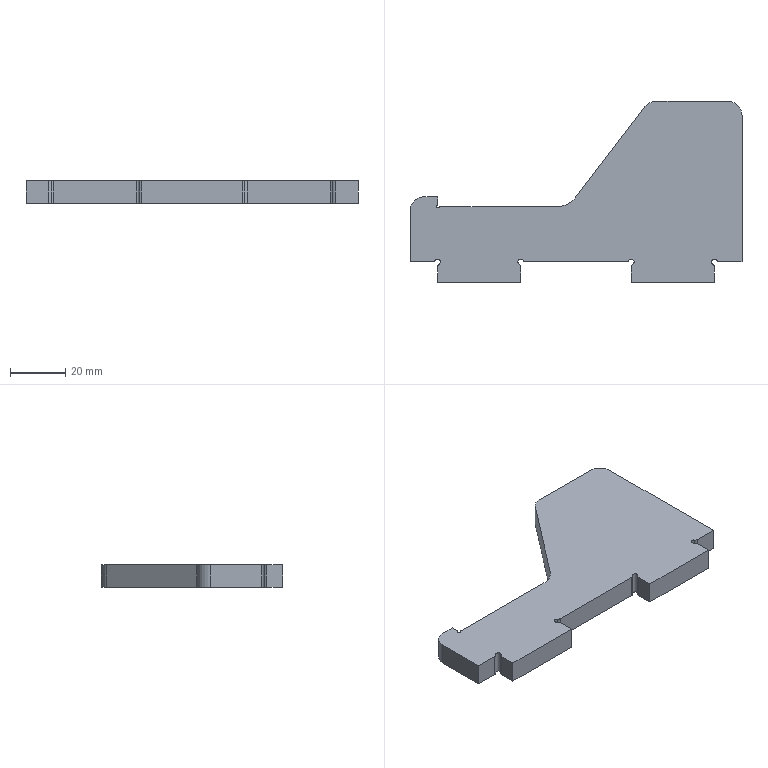Part | SolidWorks | features FlatPattern 1, SMBaseFlange 1, SheetMetal 1 | 1 solid | 39 faces | box 120 x 65.5 x 8 mm | volume 37548 mm3 | cylinder 21 | plane 18 | commonest cylinder face diameters 2 x16 10 x3 1 x1 16 x1
STEP:
#1=CARTESIAN_POINT('',(-85.366,-78.6,-8.));
#2=VERTEX_POINT('',#1);
#3=CARTESIAN_POINT('',(-83.5,-79.1,-8.));
#4=VERTEX_POINT('',#3);
#5=CARTESIAN_POINT('',(-84.5,-79.1,-8.));
#6=DIRECTION('',(0.,0.,-1.));
#7=DIRECTION('',(1.,0.,0.));
#8=AXIS2_PLACEMENT_3D('',#5,#6,#7);
#9=CIRCLE('',#8,1.);
#10=EDGE_CURVE('',#2,#4,#9,.T.);
#11=ORIENTED_EDGE('',*,*,#10,.T.);
#12=CARTESIAN_POINT('',(-83.5,-79.1,0.));
#13=VERTEX_POINT('',#12);
#14=CARTESIAN_POINT('',(-83.5,-79.1,-8.));
#15=DIRECTION('',(0.,0.,1.));
#16=VECTOR('',#15,1000.);
#17=LINE('',#14,#16);
#18=EDGE_CURVE('',#4,#13,#17,.T.);
#19=ORIENTED_EDGE('',*,*,#18,.T.);
#20=CARTESIAN_POINT('',(-85.366,-78.6,0.));
#21=VERTEX_POINT('',#20);
#22=CARTESIAN_POINT('',(-84.5,-79.1,0.));
#23=DIRECTION('',(0.,0.,-1.));
#24=DIRECTION('',(1.,0.,0.));
#25=AXIS2_PLACEMENT_3D('',#22,#23,#24);
#26=CIRCLE('',#25,1.);
#27=EDGE_CURVE('',#21,#13,#26,.T.);
#28=ORIENTED_EDGE('',*,*,#27,.F.);
#29=CARTESIAN_POINT('',(-85.366,-78.6,-8.));
#30=DIRECTION('',(0.,0.,1.));
#31=VECTOR('',#30,1000.);
#32=LINE('',#29,#31);
#33=EDGE_CURVE('',#2,#21,#32,.T.);
#34=ORIENTED_EDGE('',*,*,#33,.F.);
#35=EDGE_LOOP('',(#11,#19,#28,#34));
#36=FACE_OUTER_BOUND('',#35,.T.);
#37=CARTESIAN_POINT('',(-84.5,-79.1,-8.));
#38=DIRECTION('',(0.,0.,1.));
#39=DIRECTION('',(1.,0.,0.));
#40=AXIS2_PLACEMENT_3D('',#37,#38,#39);
#41=CYLINDRICAL_SURFACE('',#40,1.);
#42=ADVANCED_FACE('',(#36),#41,.F.);
#43=CARTESIAN_POINT('',(-15.366,-78.6,-8.));
#44=VERTEX_POINT('',#43);
#45=CARTESIAN_POINT('',(-13.5,-79.1,-8.));
#46=VERTEX_POINT('',#45);
#47=CARTESIAN_POINT('',(-14.5,-79.1,-8.));
#48=DIRECTION('',(0.,0.,-1.));
#49=DIRECTION('',(1.,0.,0.));
#50=AXIS2_PLACEMENT_3D('',#47,#48,#49);
#51=CIRCLE('',#50,1.);
#52=EDGE_CURVE('',#44,#46,#51,.T.);
#53=ORIENTED_EDGE('',*,*,#52,.T.);
#54=CARTESIAN_POINT('',(-13.5,-79.1,0.));
#55=VERTEX_POINT('',#54);
#56=CARTESIAN_POINT('',(-13.5,-79.1,-8.));
#57=DIRECTION('',(0.,0.,1.));
#58=VECTOR('',#57,1000.);
#59=LINE('',#56,#58);
#60=EDGE_CURVE('',#46,#55,#59,.T.);
#61=ORIENTED_EDGE('',*,*,#60,.T.);
#62=CARTESIAN_POINT('',(-15.366,-78.6,0.));
#63=VERTEX_POINT('',#62);
#64=CARTESIAN_POINT('',(-14.5,-79.1,0.));
#65=DIRECTION('',(0.,0.,-1.));
#66=DIRECTION('',(1.,0.,0.));
#67=AXIS2_PLACEMENT_3D('',#64,#65,#66);
#68=CIRCLE('',#67,1.);
#69=EDGE_CURVE('',#63,#55,#68,.T.);
#70=ORIENTED_EDGE('',*,*,#69,.F.);
#71=CARTESIAN_POINT('',(-15.366,-78.6,-8.));
#72=DIRECTION('',(0.,0.,1.));
#73=VECTOR('',#72,1000.);
#74=LINE('',#71,#73);
#75=EDGE_CURVE('',#44,#63,#74,.T.);
#76=ORIENTED_EDGE('',*,*,#75,.F.);
#77=EDGE_LOOP('',(#53,#61,#70,#76));
#78=FACE_OUTER_BOUND('',#77,.T.);
#79=CARTESIAN_POINT('',(-14.5,-79.1,-8.));
#80=DIRECTION('',(0.,0.,1.));
#81=DIRECTION('',(1.,0.,0.));
#82=AXIS2_PLACEMENT_3D('',#79,#80,#81);
#83=CYLINDRICAL_SURFACE('',#82,1.);
#84=ADVANCED_FACE('',(#78),#83,.F.);
#85=CARTESIAN_POINT('',(17.232,-79.1,0.));
#86=VERTEX_POINT('',#85);
#87=CARTESIAN_POINT('',(25.5,-79.1,0.));
#88=VERTEX_POINT('',#87);
#89=CARTESIAN_POINT('',(25.5,-79.1,0.));
#90=DIRECTION('',(1.,0.,0.));
#91=VECTOR('',#90,1000.);
#92=LINE('',#89,#91);
#93=EDGE_CURVE('',#86,#88,#92,.T.);
#94=ORIENTED_EDGE('',*,*,#93,.F.);
#95=CARTESIAN_POINT('',(17.232,-79.1,-8.));
#96=VERTEX_POINT('',#95);
#97=CARTESIAN_POINT('',(17.232,-79.1,-8.));
#98=DIRECTION('',(0.,0.,1.));
#99=VECTOR('',#98,1000.);
#100=LINE('',#97,#99);
#101=EDGE_CURVE('',#96,#86,#100,.T.);
#102=ORIENTED_EDGE('',*,*,#101,.F.);
#103=CARTESIAN_POINT('',(25.5,-79.1,-8.));
#104=VERTEX_POINT('',#103);
#105=CARTESIAN_POINT('',(25.5,-79.1,-8.));
#106=DIRECTION('',(1.,0.,0.));
#107=VECTOR('',#106,1000.);
#108=LINE('',#105,#107);
#109=EDGE_CURVE('',#96,#104,#108,.T.);
#110=ORIENTED_EDGE('',*,*,#109,.T.);
#111=CARTESIAN_POINT('',(25.5,-79.1,-8.));
#112=DIRECTION('',(0.,0.,1.));
#113=VECTOR('',#112,1000.);
#114=LINE('',#111,#113);
#115=EDGE_CURVE('',#104,#88,#114,.T.);
#116=ORIENTED_EDGE('',*,*,#115,.T.);
#117=EDGE_LOOP('',(#94,#102,#110,#116));
#118=FACE_OUTER_BOUND('',#117,.T.);
#119=CARTESIAN_POINT('',(25.5,-79.1,-8.));
#120=DIRECTION('',(0.,-1.,0.));
#121=DIRECTION('',(0.,0.,-1.));
#122=AXIS2_PLACEMENT_3D('',#119,#120,#121);
#123=PLANE('',#122);
#124=ADVANCED_FACE('',(#118),#123,.T.);
#125=CARTESIAN_POINT('',(16.366,-78.6,0.));
#126=VERTEX_POINT('',#125);
#127=CARTESIAN_POINT('',(17.232,-78.1,0.));
#128=DIRECTION('',(0.,0.,1.));
#129=DIRECTION('',(1.,0.,0.));
#130=AXIS2_PLACEMENT_3D('',#127,#128,#129);
#131=CIRCLE('',#130,1.);
#132=EDGE_CURVE('',#126,#86,#131,.T.);
#133=ORIENTED_EDGE('',*,*,#132,.F.);
#134=CARTESIAN_POINT('',(16.366,-78.6,-8.));
#135=VERTEX_POINT('',#134);
#136=CARTESIAN_POINT('',(16.366,-78.6,-8.));
#137=DIRECTION('',(0.,0.,1.));
#138=VECTOR('',#137,1000.);
#139=LINE('',#136,#138);
#140=EDGE_CURVE('',#135,#126,#139,.T.);
#141=ORIENTED_EDGE('',*,*,#140,.F.);
#142=CARTESIAN_POINT('',(17.232,-78.1,-8.));
#143=DIRECTION('',(0.,0.,1.));
#144=DIRECTION('',(1.,0.,0.));
#145=AXIS2_PLACEMENT_3D('',#142,#143,#144);
#146=CIRCLE('',#145,1.);
#147=EDGE_CURVE('',#135,#96,#146,.T.);
#148=ORIENTED_EDGE('',*,*,#147,.T.);
#149=ORIENTED_EDGE('',*,*,#101,.T.);
#150=EDGE_LOOP('',(#133,#141,#148,#149));
#151=FACE_OUTER_BOUND('',#150,.T.);
#152=CARTESIAN_POINT('',(17.232,-78.1,-8.));
#153=DIRECTION('',(0.,0.,1.));
#154=DIRECTION('',(1.,0.,0.));
#155=AXIS2_PLACEMENT_3D('',#152,#153,#154);
#156=CYLINDRICAL_SURFACE('',#155,1.);
#157=ADVANCED_FACE('',(#151),#156,.T.);
#158=CARTESIAN_POINT('',(15.,-79.966,0.));
#159=VERTEX_POINT('',#158);
#160=CARTESIAN_POINT('',(15.5,-79.1,0.));
#161=DIRECTION('',(0.,0.,-1.));
#162=DIRECTION('',(1.,0.,0.));
#163=AXIS2_PLACEMENT_3D('',#160,#161,#162);
#164=CIRCLE('',#163,1.);
#165=EDGE_CURVE('',#159,#126,#164,.T.);
#166=ORIENTED_EDGE('',*,*,#165,.F.);
#167=CARTESIAN_POINT('',(15.,-79.966,-8.));
#168=VERTEX_POINT('',#167);
#169=CARTESIAN_POINT('',(15.,-79.966,-8.));
#170=DIRECTION('',(0.,0.,1.));
#171=VECTOR('',#170,1000.);
#172=LINE('',#169,#171);
#173=EDGE_CURVE('',#168,#159,#172,.T.);
#174=ORIENTED_EDGE('',*,*,#173,.F.);
#175=CARTESIAN_POINT('',(15.5,-79.1,-8.));
#176=DIRECTION('',(0.,0.,-1.));
#177=DIRECTION('',(1.,0.,0.));
#178=AXIS2_PLACEMENT_3D('',#175,#176,#177);
#179=CIRCLE('',#178,1.);
#180=EDGE_CURVE('',#168,#135,#179,.T.);
#181=ORIENTED_EDGE('',*,*,#180,.T.);
#182=ORIENTED_EDGE('',*,*,#140,.T.);
#183=EDGE_LOOP('',(#166,#174,#181,#182));
#184=FACE_OUTER_BOUND('',#183,.T.);
#185=CARTESIAN_POINT('',(15.5,-79.1,-8.));
#186=DIRECTION('',(0.,0.,1.));
#187=DIRECTION('',(1.,0.,0.));
#188=AXIS2_PLACEMENT_3D('',#185,#186,#187);
#189=CYLINDRICAL_SURFACE('',#188,1.);
#190=ADVANCED_FACE('',(#184),#189,.F.);
#191=CARTESIAN_POINT('',(15.5,-80.832,0.));
#192=VERTEX_POINT('',#191);
#193=CARTESIAN_POINT('',(14.5,-80.832,0.));
#194=DIRECTION('',(0.,0.,1.));
#195=DIRECTION('',(-1.,0.,0.));
#196=AXIS2_PLACEMENT_3D('',#193,#194,#195);
#197=CIRCLE('',#196,1.);
#198=EDGE_CURVE('',#192,#159,#197,.T.);
#199=ORIENTED_EDGE('',*,*,#198,.F.);
#200=CARTESIAN_POINT('',(15.5,-80.832,-8.));
#201=VERTEX_POINT('',#200);
#202=CARTESIAN_POINT('',(15.5,-80.832,-8.));
#203=DIRECTION('',(0.,0.,1.));
#204=VECTOR('',#203,1000.);
#205=LINE('',#202,#204);
#206=EDGE_CURVE('',#201,#192,#205,.T.);
#207=ORIENTED_EDGE('',*,*,#206,.F.);
#208=CARTESIAN_POINT('',(14.5,-80.832,-8.));
#209=DIRECTION('',(0.,0.,1.));
#210=DIRECTION('',(-1.,0.,0.));
#211=AXIS2_PLACEMENT_3D('',#208,#209,#210);
#212=CIRCLE('',#211,1.);
#213=EDGE_CURVE('',#201,#168,#212,.T.);
#214=ORIENTED_EDGE('',*,*,#213,.T.);
#215=ORIENTED_EDGE('',*,*,#173,.T.);
#216=EDGE_LOOP('',(#199,#207,#214,#215));
#217=FACE_OUTER_BOUND('',#216,.T.);
#218=CARTESIAN_POINT('',(14.5,-80.832,-8.));
#219=DIRECTION('',(0.,0.,1.));
#220=DIRECTION('',(1.,0.,0.));
#221=AXIS2_PLACEMENT_3D('',#218,#219,#220);
#222=CYLINDRICAL_SURFACE('',#221,1.);
#223=ADVANCED_FACE('',(#217),#222,.T.);
#224=CARTESIAN_POINT('',(15.5,-86.6,0.));
#225=VERTEX_POINT('',#224);
#226=CARTESIAN_POINT('',(15.5,-86.6,0.));
#227=DIRECTION('',(0.,1.,0.));
#228=VECTOR('',#227,1000.);
#229=LINE('',#226,#228);
#230=EDGE_CURVE('',#225,#192,#229,.T.);
#231=ORIENTED_EDGE('',*,*,#230,.F.);
#232=CARTESIAN_POINT('',(15.5,-86.6,-8.));
#233=VERTEX_POINT('',#232);
#234=CARTESIAN_POINT('',(15.5,-86.6,-8.));
#235=DIRECTION('',(0.,0.,1.));
#236=VECTOR('',#235,1000.);
#237=LINE('',#234,#236);
#238=EDGE_CURVE('',#233,#225,#237,.T.);
#239=ORIENTED_EDGE('',*,*,#238,.F.);
#240=CARTESIAN_POINT('',(15.5,-86.6,-8.));
#241=DIRECTION('',(0.,1.,0.));
#242=VECTOR('',#241,1000.);
#243=LINE('',#240,#242);
#244=EDGE_CURVE('',#233,#201,#243,.T.);
#245=ORIENTED_EDGE('',*,*,#244,.T.);
#246=ORIENTED_EDGE('',*,*,#206,.T.);
#247=EDGE_LOOP('',(#231,#239,#245,#246));
#248=FACE_OUTER_BOUND('',#247,.T.);
#249=CARTESIAN_POINT('',(15.5,-86.6,-8.));
#250=DIRECTION('',(1.,0.,0.));
#251=DIRECTION('',(0.,1.,0.));
#252=AXIS2_PLACEMENT_3D('',#249,#250,#251);
#253=PLANE('',#252);
#254=ADVANCED_FACE('',(#248),#253,.T.);
#255=CARTESIAN_POINT('',(-14.5,-86.6,0.));
#256=VERTEX_POINT('',#255);
#257=CARTESIAN_POINT('',(-14.5,-86.6,0.));
#258=DIRECTION('',(1.,0.,0.));
#259=VECTOR('',#258,1000.);
#260=LINE('',#257,#259);
#261=EDGE_CURVE('',#256,#225,#260,.T.);
#262=ORIENTED_EDGE('',*,*,#261,.F.);
#263=CARTESIAN_POINT('',(-14.5,-86.6,-8.));
#264=VERTEX_POINT('',#263);
#265=CARTESIAN_POINT('',(-14.5,-86.6,-8.));
#266=DIRECTION('',(0.,0.,1.));
#267=VECTOR('',#266,1000.);
#268=LINE('',#265,#267);
#269=EDGE_CURVE('',#264,#256,#268,.T.);
#270=ORIENTED_EDGE('',*,*,#269,.F.);
#271=CARTESIAN_POINT('',(-14.5,-86.6,-8.));
#272=DIRECTION('',(1.,0.,0.));
#273=VECTOR('',#272,1000.);
#274=LINE('',#271,#273);
#275=EDGE_CURVE('',#264,#233,#274,.T.);
#276=ORIENTED_EDGE('',*,*,#275,.T.);
#277=ORIENTED_EDGE('',*,*,#238,.T.);
#278=EDGE_LOOP('',(#262,#270,#276,#277));
#279=FACE_OUTER_BOUND('',#278,.T.);
#280=CARTESIAN_POINT('',(-14.5,-86.6,-8.));
#281=DIRECTION('',(0.,-1.,0.));
#282=DIRECTION('',(0.,0.,-1.));
#283=AXIS2_PLACEMENT_3D('',#280,#281,#282);
#284=PLANE('',#283);
#285=ADVANCED_FACE('',(#279),#284,.T.);
#286=CARTESIAN_POINT('',(-14.5,-80.832,0.));
#287=VERTEX_POINT('',#286);
#288=CARTESIAN_POINT('',(-14.5,-80.832,0.));
#289=DIRECTION('',(0.,-1.,0.));
#290=VECTOR('',#289,1000.);
#291=LINE('',#288,#290);
#292=EDGE_CURVE('',#287,#256,#291,.T.);
#293=ORIENTED_EDGE('',*,*,#292,.F.);
#294=CARTESIAN_POINT('',(-14.5,-80.832,-8.));
#295=VERTEX_POINT('',#294);
#296=CARTESIAN_POINT('',(-14.5,-80.832,-8.));
#297=DIRECTION('',(0.,0.,1.));
#298=VECTOR('',#297,1000.);
#299=LINE('',#296,#298);
#300=EDGE_CURVE('',#295,#287,#299,.T.);
#301=ORIENTED_EDGE('',*,*,#300,.F.);
#302=CARTESIAN_POINT('',(-14.5,-80.832,-8.));
#303=DIRECTION('',(0.,-1.,0.));
#304=VECTOR('',#303,1000.);
#305=LINE('',#302,#304);
#306=EDGE_CURVE('',#295,#264,#305,.T.);
#307=ORIENTED_EDGE('',*,*,#306,.T.);
#308=ORIENTED_EDGE('',*,*,#269,.T.);
#309=EDGE_LOOP('',(#293,#301,#307,#308));
#310=FACE_OUTER_BOUND('',#309,.T.);
#311=CARTESIAN_POINT('',(-14.5,-80.832,-8.));
#312=DIRECTION('',(-1.,0.,0.));
#313=DIRECTION('',(0.,0.,1.));
#314=AXIS2_PLACEMENT_3D('',#311,#312,#313);
#315=PLANE('',#314);
#316=ADVANCED_FACE('',(#310),#315,.T.);
#317=CARTESIAN_POINT('',(-14.,-79.966,0.));
#318=VERTEX_POINT('',#317);
#319=CARTESIAN_POINT('',(-13.5,-80.832,0.));
#320=DIRECTION('',(0.,0.,1.));
#321=DIRECTION('',(1.,0.,0.));
#322=AXIS2_PLACEMENT_3D('',#319,#320,#321);
#323=CIRCLE('',#322,1.);
#324=EDGE_CURVE('',#318,#287,#323,.T.);
#325=ORIENTED_EDGE('',*,*,#324,.F.);
#326=CARTESIAN_POINT('',(-14.,-79.966,-8.));
#327=VERTEX_POINT('',#326);
#328=CARTESIAN_POINT('',(-14.,-79.966,-8.));
#329=DIRECTION('',(0.,0.,1.));
#330=VECTOR('',#329,1000.);
#331=LINE('',#328,#330);
#332=EDGE_CURVE('',#327,#318,#331,.T.);
#333=ORIENTED_EDGE('',*,*,#332,.F.);
#334=CARTESIAN_POINT('',(-13.5,-80.832,-8.));
#335=DIRECTION('',(0.,0.,1.));
#336=DIRECTION('',(1.,0.,0.));
#337=AXIS2_PLACEMENT_3D('',#334,#335,#336);
#338=CIRCLE('',#337,1.);
#339=EDGE_CURVE('',#327,#295,#338,.T.);
#340=ORIENTED_EDGE('',*,*,#339,.T.);
#341=ORIENTED_EDGE('',*,*,#300,.T.);
#342=EDGE_LOOP('',(#325,#333,#340,#341));
#343=FACE_OUTER_BOUND('',#342,.T.);
#344=CARTESIAN_POINT('',(-13.5,-80.832,-8.));
#345=DIRECTION('',(0.,0.,1.));
#346=DIRECTION('',(1.,0.,0.));
#347=AXIS2_PLACEMENT_3D('',#344,#345,#346);
#348=CYLINDRICAL_SURFACE('',#347,1.);
#349=ADVANCED_FACE('',(#343),#348,.T.);
#350=ORIENTED_EDGE('',*,*,#60,.F.);
#351=CARTESIAN_POINT('',(-14.5,-79.1,-8.));
#352=DIRECTION('',(0.,0.,-1.));
#353=DIRECTION('',(1.,0.,0.));
#354=AXIS2_PLACEMENT_3D('',#351,#352,#353);
#355=CIRCLE('',#354,1.);
#356=EDGE_CURVE('',#46,#327,#355,.T.);
#357=ORIENTED_EDGE('',*,*,#356,.T.);
#358=ORIENTED_EDGE('',*,*,#332,.T.);
#359=CARTESIAN_POINT('',(-14.5,-79.1,0.));
#360=DIRECTION('',(0.,0.,-1.));
#361=DIRECTION('',(1.,0.,0.));
#362=AXIS2_PLACEMENT_3D('',#359,#360,#361);
#363=CIRCLE('',#362,1.);
#364=EDGE_CURVE('',#55,#318,#363,.T.);
#365=ORIENTED_EDGE('',*,*,#364,.F.);
#366=EDGE_LOOP('',(#350,#357,#358,#365));
#367=FACE_OUTER_BOUND('',#366,.T.);
#368=CARTESIAN_POINT('',(-14.5,-79.1,-8.));
#369=DIRECTION('',(0.,0.,1.));
#370=DIRECTION('',(1.,0.,0.));
#371=AXIS2_PLACEMENT_3D('',#368,#369,#370);
#372=CYLINDRICAL_SURFACE('',#371,1.);
#373=ADVANCED_FACE('',(#367),#372,.F.);
#374=CARTESIAN_POINT('',(-16.232,-79.1,0.));
#375=VERTEX_POINT('',#374);
#376=CARTESIAN_POINT('',(-16.232,-78.1,0.));
#377=DIRECTION('',(0.,0.,1.));
#378=DIRECTION('',(-1.,0.,0.));
#379=AXIS2_PLACEMENT_3D('',#376,#377,#378);
#380=CIRCLE('',#379,1.);
#381=EDGE_CURVE('',#375,#63,#380,.T.);
#382=ORIENTED_EDGE('',*,*,#381,.F.);
#383=CARTESIAN_POINT('',(-16.232,-79.1,-8.));
#384=VERTEX_POINT('',#383);
#385=CARTESIAN_POINT('',(-16.232,-79.1,-8.));
#386=DIRECTION('',(0.,0.,1.));
#387=VECTOR('',#386,1000.);
#388=LINE('',#385,#387);
#389=EDGE_CURVE('',#384,#375,#388,.T.);
#390=ORIENTED_EDGE('',*,*,#389,.F.);
#391=CARTESIAN_POINT('',(-16.232,-78.1,-8.));
#392=DIRECTION('',(0.,0.,1.));
#393=DIRECTION('',(-1.,0.,0.));
#394=AXIS2_PLACEMENT_3D('',#391,#392,#393);
#395=CIRCLE('',#394,1.);
#396=EDGE_CURVE('',#384,#44,#395,.T.);
#397=ORIENTED_EDGE('',*,*,#396,.T.);
#398=ORIENTED_EDGE('',*,*,#75,.T.);
#399=EDGE_LOOP('',(#382,#390,#397,#398));
#400=FACE_OUTER_BOUND('',#399,.T.);
#401=CARTESIAN_POINT('',(-16.232,-78.1,-8.));
#402=DIRECTION('',(0.,0.,1.));
#403=DIRECTION('',(1.,0.,0.));
#404=AXIS2_PLACEMENT_3D('',#401,#402,#403);
#405=CYLINDRICAL_SURFACE('',#404,1.);
#406=ADVANCED_FACE('',(#400),#405,.T.);
#407=CARTESIAN_POINT('',(-52.768,-79.1,0.));
#408=VERTEX_POINT('',#407);
#409=CARTESIAN_POINT('',(-16.232,-79.1,0.));
#410=DIRECTION('',(1.,0.,0.));
#411=VECTOR('',#410,1000.);
#412=LINE('',#409,#411);
#413=EDGE_CURVE('',#408,#375,#412,.T.);
#414=ORIENTED_EDGE('',*,*,#413,.F.);
#415=CARTESIAN_POINT('',(-52.768,-79.1,-8.));
#416=VERTEX_POINT('',#415);
#417=CARTESIAN_POINT('',(-52.768,-79.1,-8.));
#418=DIRECTION('',(0.,0.,1.));
#419=VECTOR('',#418,1000.);
#420=LINE('',#417,#419);
#421=EDGE_CURVE('',#416,#408,#420,.T.);
#422=ORIENTED_EDGE('',*,*,#421,.F.);
#423=CARTESIAN_POINT('',(-16.232,-79.1,-8.));
#424=DIRECTION('',(1.,0.,0.));
#425=VECTOR('',#424,1000.);
#426=LINE('',#423,#425);
#427=EDGE_CURVE('',#416,#384,#426,.T.);
#428=ORIENTED_EDGE('',*,*,#427,.T.);
#429=ORIENTED_EDGE('',*,*,#389,.T.);
#430=EDGE_LOOP('',(#414,#422,#428,#429));
#431=FACE_OUTER_BOUND('',#430,.T.);
#432=CARTESIAN_POINT('',(-16.232,-79.1,-8.));
#433=DIRECTION('',(0.,-1.,0.));
#434=DIRECTION('',(1.,0.,0.));
#435=AXIS2_PLACEMENT_3D('',#432,#433,#434);
#436=PLANE('',#435);
#437=ADVANCED_FACE('',(#431),#436,.T.);
#438=CARTESIAN_POINT('',(-53.634,-78.6,0.));
#439=VERTEX_POINT('',#438);
#440=CARTESIAN_POINT('',(-52.768,-78.1,0.));
#441=DIRECTION('',(0.,0.,1.));
#442=DIRECTION('',(1.,0.,0.));
#443=AXIS2_PLACEMENT_3D('',#440,#441,#442);
#444=CIRCLE('',#443,1.);
#445=EDGE_CURVE('',#439,#408,#444,.T.);
#446=ORIENTED_EDGE('',*,*,#445,.F.);
#447=CARTESIAN_POINT('',(-53.634,-78.6,-8.));
#448=VERTEX_POINT('',#447);
#449=CARTESIAN_POINT('',(-53.634,-78.6,-8.));
#450=DIRECTION('',(0.,0.,1.));
#451=VECTOR('',#450,1000.);
#452=LINE('',#449,#451);
#453=EDGE_CURVE('',#448,#439,#452,.T.);
#454=ORIENTED_EDGE('',*,*,#453,.F.);
#455=CARTESIAN_POINT('',(-52.768,-78.1,-8.));
#456=DIRECTION('',(0.,0.,1.));
#457=DIRECTION('',(1.,0.,0.));
#458=AXIS2_PLACEMENT_3D('',#455,#456,#457);
#459=CIRCLE('',#458,1.);
#460=EDGE_CURVE('',#448,#416,#459,.T.);
#461=ORIENTED_EDGE('',*,*,#460,.T.);
#462=ORIENTED_EDGE('',*,*,#421,.T.);
#463=EDGE_LOOP('',(#446,#454,#461,#462));
#464=FACE_OUTER_BOUND('',#463,.T.);
#465=CARTESIAN_POINT('',(-52.768,-78.1,-8.));
#466=DIRECTION('',(0.,0.,1.));
#467=DIRECTION('',(1.,0.,0.));
#468=AXIS2_PLACEMENT_3D('',#465,#466,#467);
#469=CYLINDRICAL_SURFACE('',#468,1.);
#470=ADVANCED_FACE('',(#464),#469,.T.);
#471=CARTESIAN_POINT('',(-55.,-79.966,0.));
#472=VERTEX_POINT('',#471);
#473=CARTESIAN_POINT('',(-54.5,-79.1,0.));
#474=DIRECTION('',(0.,0.,-1.));
#475=DIRECTION('',(1.,0.,0.));
#476=AXIS2_PLACEMENT_3D('',#473,#474,#475);
#477=CIRCLE('',#476,1.);
#478=EDGE_CURVE('',#472,#439,#477,.T.);
#479=ORIENTED_EDGE('',*,*,#478,.F.);
#480=CARTESIAN_POINT('',(-55.,-79.966,-8.));
#481=VERTEX_POINT('',#480);
#482=CARTESIAN_POINT('',(-55.,-79.966,-8.));
#483=DIRECTION('',(0.,0.,1.));
#484=VECTOR('',#483,1000.);
#485=LINE('',#482,#484);
#486=EDGE_CURVE('',#481,#472,#485,.T.);
#487=ORIENTED_EDGE('',*,*,#486,.F.);
#488=CARTESIAN_POINT('',(-54.5,-79.1,-8.));
#489=DIRECTION('',(0.,0.,-1.));
#490=DIRECTION('',(1.,0.,0.));
#491=AXIS2_PLACEMENT_3D('',#488,#489,#490);
#492=CIRCLE('',#491,1.);
#493=EDGE_CURVE('',#481,#448,#492,.T.);
#494=ORIENTED_EDGE('',*,*,#493,.T.);
#495=ORIENTED_EDGE('',*,*,#453,.T.);
#496=EDGE_LOOP('',(#479,#487,#494,#495));
#497=FACE_OUTER_BOUND('',#496,.T.);
#498=CARTESIAN_POINT('',(-54.5,-79.1,-8.));
#499=DIRECTION('',(0.,0.,1.));
#500=DIRECTION('',(1.,0.,0.));
#501=AXIS2_PLACEMENT_3D('',#498,#499,#500);
#502=CYLINDRICAL_SURFACE('',#501,1.);
#503=ADVANCED_FACE('',(#497),#502,.F.);
#504=CARTESIAN_POINT('',(-54.5,-80.832,0.));
#505=VERTEX_POINT('',#504);
#506=CARTESIAN_POINT('',(-55.5,-80.832,0.));
#507=DIRECTION('',(0.,0.,1.));
#508=DIRECTION('',(-1.,0.,0.));
#509=AXIS2_PLACEMENT_3D('',#506,#507,#508);
#510=CIRCLE('',#509,1.);
#511=EDGE_CURVE('',#505,#472,#510,.T.);
#512=ORIENTED_EDGE('',*,*,#511,.F.);
#513=CARTESIAN_POINT('',(-54.5,-80.832,-8.));
#514=VERTEX_POINT('',#513);
#515=CARTESIAN_POINT('',(-54.5,-80.832,-8.));
#516=DIRECTION('',(0.,0.,1.));
#517=VECTOR('',#516,1000.);
#518=LINE('',#515,#517);
#519=EDGE_CURVE('',#514,#505,#518,.T.);
#520=ORIENTED_EDGE('',*,*,#519,.F.);
#521=CARTESIAN_POINT('',(-55.5,-80.832,-8.));
#522=DIRECTION('',(0.,0.,1.));
#523=DIRECTION('',(-1.,0.,0.));
#524=AXIS2_PLACEMENT_3D('',#521,#522,#523);
#525=CIRCLE('',#524,1.);
#526=EDGE_CURVE('',#514,#481,#525,.T.);
#527=ORIENTED_EDGE('',*,*,#526,.T.);
#528=ORIENTED_EDGE('',*,*,#486,.T.);
#529=EDGE_LOOP('',(#512,#520,#527,#528));
#530=FACE_OUTER_BOUND('',#529,.T.);
#531=CARTESIAN_POINT('',(-55.5,-80.832,-8.));
#532=DIRECTION('',(0.,0.,1.));
#533=DIRECTION('',(1.,0.,0.));
#534=AXIS2_PLACEMENT_3D('',#531,#532,#533);
#535=CYLINDRICAL_SURFACE('',#534,1.);
#536=ADVANCED_FACE('',(#530),#535,.T.);
#537=CARTESIAN_POINT('',(-54.5,-86.6,0.));
#538=VERTEX_POINT('',#537);
#539=CARTESIAN_POINT('',(-54.5,-86.6,0.));
#540=DIRECTION('',(0.,1.,0.));
#541=VECTOR('',#540,1000.);
#542=LINE('',#539,#541);
#543=EDGE_CURVE('',#538,#505,#542,.T.);
#544=ORIENTED_EDGE('',*,*,#543,.F.);
#545=CARTESIAN_POINT('',(-54.5,-86.6,-8.));
#546=VERTEX_POINT('',#545);
#547=CARTESIAN_POINT('',(-54.5,-86.6,-8.));
#548=DIRECTION('',(0.,0.,1.));
#549=VECTOR('',#548,1000.);
#550=LINE('',#547,#549);
#551=EDGE_CURVE('',#546,#538,#550,.T.);
#552=ORIENTED_EDGE('',*,*,#551,.F.);
#553=CARTESIAN_POINT('',(-54.5,-86.6,-8.));
#554=DIRECTION('',(0.,1.,0.));
#555=VECTOR('',#554,1000.);
#556=LINE('',#553,#555);
#557=EDGE_CURVE('',#546,#514,#556,.T.);
#558=ORIENTED_EDGE('',*,*,#557,.T.);
#559=ORIENTED_EDGE('',*,*,#519,.T.);
#560=EDGE_LOOP('',(#544,#552,#558,#559));
#561=FACE_OUTER_BOUND('',#560,.T.);
#562=CARTESIAN_POINT('',(-54.5,-86.6,-8.));
#563=DIRECTION('',(1.,0.,0.));
#564=DIRECTION('',(0.,0.,-1.));
#565=AXIS2_PLACEMENT_3D('',#562,#563,#564);
#566=PLANE('',#565);
#567=ADVANCED_FACE('',(#561),#566,.T.);
#568=CARTESIAN_POINT('',(-84.5,-86.6,0.));
#569=VERTEX_POINT('',#568);
#570=CARTESIAN_POINT('',(-84.5,-86.6,0.));
#571=DIRECTION('',(1.,0.,0.));
#572=VECTOR('',#571,1000.);
#573=LINE('',#570,#572);
#574=EDGE_CURVE('',#569,#538,#573,.T.);
#575=ORIENTED_EDGE('',*,*,#574,.F.);
#576=CARTESIAN_POINT('',(-84.5,-86.6,-8.));
#577=VERTEX_POINT('',#576);
#578=CARTESIAN_POINT('',(-84.5,-86.6,-8.));
#579=DIRECTION('',(0.,0.,1.));
#580=VECTOR('',#579,1000.);
#581=LINE('',#578,#580);
#582=EDGE_CURVE('',#577,#569,#581,.T.);
#583=ORIENTED_EDGE('',*,*,#582,.F.);
#584=CARTESIAN_POINT('',(-84.5,-86.6,-8.));
#585=DIRECTION('',(1.,0.,0.));
#586=VECTOR('',#585,1000.);
#587=LINE('',#584,#586);
#588=EDGE_CURVE('',#577,#546,#587,.T.);
#589=ORIENTED_EDGE('',*,*,#588,.T.);
#590=ORIENTED_EDGE('',*,*,#551,.T.);
#591=EDGE_LOOP('',(#575,#583,#589,#590));
#592=FACE_OUTER_BOUND('',#591,.T.);
#593=CARTESIAN_POINT('',(-84.5,-86.6,-8.));
#594=DIRECTION('',(0.,-1.,0.));
#595=DIRECTION('',(0.,0.,-1.));
#596=AXIS2_PLACEMENT_3D('',#593,#594,#595);
#597=PLANE('',#596);
#598=ADVANCED_FACE('',(#592),#597,.T.);
#599=CARTESIAN_POINT('',(-84.5,-80.832,0.));
#600=VERTEX_POINT('',#599);
#601=CARTESIAN_POINT('',(-84.5,-80.832,0.));
#602=DIRECTION('',(0.,-1.,0.));
#603=VECTOR('',#602,1000.);
#604=LINE('',#601,#603);
#605=EDGE_CURVE('',#600,#569,#604,.T.);
#606=ORIENTED_EDGE('',*,*,#605,.F.);
#607=CARTESIAN_POINT('',(-84.5,-80.832,-8.));
#608=VERTEX_POINT('',#607);
#609=CARTESIAN_POINT('',(-84.5,-80.832,-8.));
#610=DIRECTION('',(0.,0.,1.));
#611=VECTOR('',#610,1000.);
#612=LINE('',#609,#611);
#613=EDGE_CURVE('',#608,#600,#612,.T.);
#614=ORIENTED_EDGE('',*,*,#613,.F.);
#615=CARTESIAN_POINT('',(-84.5,-80.832,-8.));
#616=DIRECTION('',(0.,-1.,0.));
#617=VECTOR('',#616,1000.);
#618=LINE('',#615,#617);
#619=EDGE_CURVE('',#608,#577,#618,.T.);
#620=ORIENTED_EDGE('',*,*,#619,.T.);
#621=ORIENTED_EDGE('',*,*,#582,.T.);
#622=EDGE_LOOP('',(#606,#614,#620,#621));
#623=FACE_OUTER_BOUND('',#622,.T.);
#624=CARTESIAN_POINT('',(-84.5,-80.832,-8.));
#625=DIRECTION('',(-1.,0.,0.));
#626=DIRECTION('',(0.,0.,1.));
#627=AXIS2_PLACEMENT_3D('',#624,#625,#626);
#628=PLANE('',#627);
#629=ADVANCED_FACE('',(#623),#628,.T.);
#630=CARTESIAN_POINT('',(-84.,-79.966,0.));
#631=VERTEX_POINT('',#630);
#632=CARTESIAN_POINT('',(-83.5,-80.832,0.));
#633=DIRECTION('',(0.,0.,1.));
#634=DIRECTION('',(1.,0.,0.));
#635=AXIS2_PLACEMENT_3D('',#632,#633,#634);
#636=CIRCLE('',#635,1.);
#637=EDGE_CURVE('',#631,#600,#636,.T.);
#638=ORIENTED_EDGE('',*,*,#637,.F.);
#639=CARTESIAN_POINT('',(-84.,-79.966,-8.));
#640=VERTEX_POINT('',#639);
#641=CARTESIAN_POINT('',(-84.,-79.966,-8.));
#642=DIRECTION('',(0.,0.,1.));
#643=VECTOR('',#642,1000.);
#644=LINE('',#641,#643);
#645=EDGE_CURVE('',#640,#631,#644,.T.);
#646=ORIENTED_EDGE('',*,*,#645,.F.);
#647=CARTESIAN_POINT('',(-83.5,-80.832,-8.));
#648=DIRECTION('',(0.,0.,1.));
#649=DIRECTION('',(1.,0.,0.));
#650=AXIS2_PLACEMENT_3D('',#647,#648,#649);
#651=CIRCLE('',#650,1.);
#652=EDGE_CURVE('',#640,#608,#651,.T.);
#653=ORIENTED_EDGE('',*,*,#652,.T.);
#654=ORIENTED_EDGE('',*,*,#613,.T.);
#655=EDGE_LOOP('',(#638,#646,#653,#654));
#656=FACE_OUTER_BOUND('',#655,.T.);
#657=CARTESIAN_POINT('',(-83.5,-80.832,-8.));
#658=DIRECTION('',(0.,0.,1.));
#659=DIRECTION('',(1.,0.,0.));
#660=AXIS2_PLACEMENT_3D('',#657,#658,#659);
#661=CYLINDRICAL_SURFACE('',#660,1.);
#662=ADVANCED_FACE('',(#656),#661,.T.);
#663=ORIENTED_EDGE('',*,*,#18,.F.);
#664=CARTESIAN_POINT('',(-84.5,-79.1,-8.));
#665=DIRECTION('',(0.,0.,-1.));
#666=DIRECTION('',(1.,0.,0.));
#667=AXIS2_PLACEMENT_3D('',#664,#665,#666);
#668=CIRCLE('',#667,1.);
#669=EDGE_CURVE('',#4,#640,#668,.T.);
#670=ORIENTED_EDGE('',*,*,#669,.T.);
#671=ORIENTED_EDGE('',*,*,#645,.T.);
#672=CARTESIAN_POINT('',(-84.5,-79.1,0.));
#673=DIRECTION('',(0.,0.,-1.));
#674=DIRECTION('',(1.,0.,0.));
#675=AXIS2_PLACEMENT_3D('',#672,#673,#674);
#676=CIRCLE('',#675,1.);
#677=EDGE_CURVE('',#13,#631,#676,.T.);
#678=ORIENTED_EDGE('',*,*,#677,.F.);
#679=EDGE_LOOP('',(#663,#670,#671,#678));
#680=FACE_OUTER_BOUND('',#679,.T.);
#681=CARTESIAN_POINT('',(-84.5,-79.1,-8.));
#682=DIRECTION('',(0.,0.,1.));
#683=DIRECTION('',(1.,0.,0.));
#684=AXIS2_PLACEMENT_3D('',#681,#682,#683);
#685=CYLINDRICAL_SURFACE('',#684,1.);
#686=ADVANCED_FACE('',(#680),#685,.F.);
#687=CARTESIAN_POINT('',(-86.232,-79.1,0.));
#688=VERTEX_POINT('',#687);
#689=CARTESIAN_POINT('',(-86.232,-78.1,0.));
#690=DIRECTION('',(0.,0.,1.));
#691=DIRECTION('',(-1.,0.,0.));
#692=AXIS2_PLACEMENT_3D('',#689,#690,#691);
#693=CIRCLE('',#692,1.);
#694=EDGE_CURVE('',#688,#21,#693,.T.);
#695=ORIENTED_EDGE('',*,*,#694,.F.);
#696=CARTESIAN_POINT('',(-86.232,-79.1,-8.));
#697=VERTEX_POINT('',#696);
#698=CARTESIAN_POINT('',(-86.232,-79.1,-8.));
#699=DIRECTION('',(0.,0.,1.));
#700=VECTOR('',#699,1000.);
#701=LINE('',#698,#700);
#702=EDGE_CURVE('',#697,#688,#701,.T.);
#703=ORIENTED_EDGE('',*,*,#702,.F.);
#704=CARTESIAN_POINT('',(-86.232,-78.1,-8.));
#705=DIRECTION('',(0.,0.,1.));
#706=DIRECTION('',(-1.,0.,0.));
#707=AXIS2_PLACEMENT_3D('',#704,#705,#706);
#708=CIRCLE('',#707,1.);
#709=EDGE_CURVE('',#697,#2,#708,.T.);
#710=ORIENTED_EDGE('',*,*,#709,.T.);
#711=ORIENTED_EDGE('',*,*,#33,.T.);
#712=EDGE_LOOP('',(#695,#703,#710,#711));
#713=FACE_OUTER_BOUND('',#712,.T.);
#714=CARTESIAN_POINT('',(-86.232,-78.1,-8.));
#715=DIRECTION('',(0.,0.,1.));
#716=DIRECTION('',(1.,0.,0.));
#717=AXIS2_PLACEMENT_3D('',#714,#715,#716);
#718=CYLINDRICAL_SURFACE('',#717,1.);
#719=ADVANCED_FACE('',(#713),#718,.T.);
#720=CARTESIAN_POINT('',(-94.5,-79.1,0.));
#721=VERTEX_POINT('',#720);
#722=CARTESIAN_POINT('',(-86.232,-79.1,0.));
#723=DIRECTION('',(1.,0.,0.));
#724=VECTOR('',#723,1000.);
#725=LINE('',#722,#724);
#726=EDGE_CURVE('',#721,#688,#725,.T.);
#727=ORIENTED_EDGE('',*,*,#726,.F.);
#728=CARTESIAN_POINT('',(-94.5,-79.1,-8.));
#729=VERTEX_POINT('',#728);
#730=CARTESIAN_POINT('',(-94.5,-79.1,-8.));
#731=DIRECTION('',(0.,0.,1.));
#732=VECTOR('',#731,1000.);
#733=LINE('',#730,#732);
#734=EDGE_CURVE('',#729,#721,#733,.T.);
#735=ORIENTED_EDGE('',*,*,#734,.F.);
#736=CARTESIAN_POINT('',(-86.232,-79.1,-8.));
#737=DIRECTION('',(1.,0.,0.));
#738=VECTOR('',#737,1000.);
#739=LINE('',#736,#738);
#740=EDGE_CURVE('',#729,#697,#739,.T.);
#741=ORIENTED_EDGE('',*,*,#740,.T.);
#742=ORIENTED_EDGE('',*,*,#702,.T.);
#743=EDGE_LOOP('',(#727,#735,#741,#742));
#744=FACE_OUTER_BOUND('',#743,.T.);
#745=CARTESIAN_POINT('',(-86.232,-79.1,-8.));
#746=DIRECTION('',(0.,-1.,0.));
#747=DIRECTION('',(0.,0.,-1.));
#748=AXIS2_PLACEMENT_3D('',#745,#746,#747);
#749=PLANE('',#748);
#750=ADVANCED_FACE('',(#744),#749,.T.);
#751=CARTESIAN_POINT('',(-94.5,-60.6,0.));
#752=VERTEX_POINT('',#751);
#753=CARTESIAN_POINT('',(-94.5,-60.6,0.));
#754=DIRECTION('',(0.,-1.,0.));
#755=VECTOR('',#754,1000.);
#756=LINE('',#753,#755);
#757=EDGE_CURVE('',#752,#721,#756,.T.);
#758=ORIENTED_EDGE('',*,*,#757,.F.);
#759=CARTESIAN_POINT('',(-94.5,-60.6,-8.));
#760=VERTEX_POINT('',#759);
#761=CARTESIAN_POINT('',(-94.5,-60.6,-8.));
#762=DIRECTION('',(0.,0.,1.));
#763=VECTOR('',#762,1000.);
#764=LINE('',#761,#763);
#765=EDGE_CURVE('',#760,#752,#764,.T.);
#766=ORIENTED_EDGE('',*,*,#765,.F.);
#767=CARTESIAN_POINT('',(-94.5,-60.6,-8.));
#768=DIRECTION('',(0.,-1.,0.));
#769=VECTOR('',#768,1000.);
#770=LINE('',#767,#769);
#771=EDGE_CURVE('',#760,#729,#770,.T.);
#772=ORIENTED_EDGE('',*,*,#771,.T.);
#773=ORIENTED_EDGE('',*,*,#734,.T.);
#774=EDGE_LOOP('',(#758,#766,#772,#773));
#775=FACE_OUTER_BOUND('',#774,.T.);
#776=CARTESIAN_POINT('',(-94.5,-60.6,-8.));
#777=DIRECTION('',(-1.,0.,0.));
#778=DIRECTION('',(0.,0.,1.));
#779=AXIS2_PLACEMENT_3D('',#776,#777,#778);
#780=PLANE('',#779);
#781=ADVANCED_FACE('',(#775),#780,.T.);
#782=CARTESIAN_POINT('',(-89.5,-55.6,0.));
#783=VERTEX_POINT('',#782);
#784=CARTESIAN_POINT('',(-89.5,-60.6,0.));
#785=DIRECTION('',(0.,0.,1.));
#786=DIRECTION('',(-1.,0.,0.));
#787=AXIS2_PLACEMENT_3D('',#784,#785,#786);
#788=CIRCLE('',#787,5.);
#789=EDGE_CURVE('',#783,#752,#788,.T.);
#790=ORIENTED_EDGE('',*,*,#789,.F.);
#791=CARTESIAN_POINT('',(-89.5,-55.6,-8.));
#792=VERTEX_POINT('',#791);
#793=CARTESIAN_POINT('',(-89.5,-55.6,-8.));
#794=DIRECTION('',(0.,0.,1.));
#795=VECTOR('',#794,1000.);
#796=LINE('',#793,#795);
#797=EDGE_CURVE('',#792,#783,#796,.T.);
#798=ORIENTED_EDGE('',*,*,#797,.F.);
#799=CARTESIAN_POINT('',(-89.5,-60.6,-8.));
#800=DIRECTION('',(0.,0.,1.));
#801=DIRECTION('',(-1.,0.,0.));
#802=AXIS2_PLACEMENT_3D('',#799,#800,#801);
#803=CIRCLE('',#802,5.);
#804=EDGE_CURVE('',#792,#760,#803,.T.);
#805=ORIENTED_EDGE('',*,*,#804,.T.);
#806=ORIENTED_EDGE('',*,*,#765,.T.);
#807=EDGE_LOOP('',(#790,#798,#805,#806));
#808=FACE_OUTER_BOUND('',#807,.T.);
#809=CARTESIAN_POINT('',(-89.5,-60.6,-8.));
#810=DIRECTION('',(0.,0.,1.));
#811=DIRECTION('',(1.,0.,0.));
#812=AXIS2_PLACEMENT_3D('',#809,#810,#811);
#813=CYLINDRICAL_SURFACE('',#812,5.);
#814=ADVANCED_FACE('',(#808),#813,.T.);
#815=CARTESIAN_POINT('',(-84.5,-55.6,0.));
#816=VERTEX_POINT('',#815);
#817=CARTESIAN_POINT('',(-84.5,-55.6,0.));
#818=DIRECTION('',(-1.,0.,0.));
#819=VECTOR('',#818,1000.);
#820=LINE('',#817,#819);
#821=EDGE_CURVE('',#816,#783,#820,.T.);
#822=ORIENTED_EDGE('',*,*,#821,.F.);
#823=CARTESIAN_POINT('',(-84.5,-55.6,-8.));
#824=VERTEX_POINT('',#823);
#825=CARTESIAN_POINT('',(-84.5,-55.6,-8.));
#826=DIRECTION('',(0.,0.,1.));
#827=VECTOR('',#826,1000.);
#828=LINE('',#825,#827);
#829=EDGE_CURVE('',#824,#816,#828,.T.);
#830=ORIENTED_EDGE('',*,*,#829,.F.);
#831=CARTESIAN_POINT('',(-84.5,-55.6,-8.));
#832=DIRECTION('',(-1.,0.,0.));
#833=VECTOR('',#832,1000.);
#834=LINE('',#831,#833);
#835=EDGE_CURVE('',#824,#792,#834,.T.);
#836=ORIENTED_EDGE('',*,*,#835,.T.);
#837=ORIENTED_EDGE('',*,*,#797,.T.);
#838=EDGE_LOOP('',(#822,#830,#836,#837));
#839=FACE_OUTER_BOUND('',#838,.T.);
#840=CARTESIAN_POINT('',(-84.5,-55.6,-8.));
#841=DIRECTION('',(0.,1.,0.));
#842=DIRECTION('',(0.,0.,1.));
#843=AXIS2_PLACEMENT_3D('',#840,#841,#842);
#844=PLANE('',#843);
#845=ADVANCED_FACE('',(#839),#844,.T.);
#846=CARTESIAN_POINT('',(-84.5,-57.982,0.));
#847=VERTEX_POINT('',#846);
#848=CARTESIAN_POINT('',(-84.5,-57.982,0.));
#849=DIRECTION('',(0.,1.,0.));
#850=VECTOR('',#849,1000.);
#851=LINE('',#848,#850);
#852=EDGE_CURVE('',#847,#816,#851,.T.);
#853=ORIENTED_EDGE('',*,*,#852,.F.);
#854=CARTESIAN_POINT('',(-84.5,-57.982,-8.));
#855=VERTEX_POINT('',#854);
#856=CARTESIAN_POINT('',(-84.5,-57.982,-8.));
#857=DIRECTION('',(0.,0.,1.));
#858=VECTOR('',#857,1000.);
#859=LINE('',#856,#858);
#860=EDGE_CURVE('',#855,#847,#859,.T.);
#861=ORIENTED_EDGE('',*,*,#860,.F.);
#862=CARTESIAN_POINT('',(-84.5,-57.982,-8.));
#863=DIRECTION('',(0.,1.,0.));
#864=VECTOR('',#863,1000.);
#865=LINE('',#862,#864);
#866=EDGE_CURVE('',#855,#824,#865,.T.);
#867=ORIENTED_EDGE('',*,*,#866,.T.);
#868=ORIENTED_EDGE('',*,*,#829,.T.);
#869=EDGE_LOOP('',(#853,#861,#867,#868));
#870=FACE_OUTER_BOUND('',#869,.T.);
#871=CARTESIAN_POINT('',(-84.5,-57.982,-8.));
#872=DIRECTION('',(1.,0.,0.));
#873=DIRECTION('',(0.,0.,-1.));
#874=AXIS2_PLACEMENT_3D('',#871,#872,#873);
#875=PLANE('',#874);
#876=ADVANCED_FACE('',(#870),#875,.T.);
#877=CARTESIAN_POINT('',(-84.833,-58.727,0.));
#878=VERTEX_POINT('',#877);
#879=CARTESIAN_POINT('',(-85.5,-57.982,0.));
#880=DIRECTION('',(0.,0.,1.));
#881=DIRECTION('',(1.,0.,0.));
#882=AXIS2_PLACEMENT_3D('',#879,#880,#881);
#883=CIRCLE('',#882,1.);
#884=EDGE_CURVE('',#878,#847,#883,.T.);
#885=ORIENTED_EDGE('',*,*,#884,.F.);
#886=CARTESIAN_POINT('',(-84.833,-58.727,-8.));
#887=VERTEX_POINT('',#886);
#888=CARTESIAN_POINT('',(-84.833,-58.727,-8.));
#889=DIRECTION('',(0.,0.,1.));
#890=VECTOR('',#889,1000.);
#891=LINE('',#888,#890);
#892=EDGE_CURVE('',#887,#878,#891,.T.);
#893=ORIENTED_EDGE('',*,*,#892,.F.);
#894=CARTESIAN_POINT('',(-85.5,-57.982,-8.));
#895=DIRECTION('',(0.,0.,1.));
#896=DIRECTION('',(1.,0.,0.));
#897=AXIS2_PLACEMENT_3D('',#894,#895,#896);
#898=CIRCLE('',#897,1.);
#899=EDGE_CURVE('',#887,#855,#898,.T.);
#900=ORIENTED_EDGE('',*,*,#899,.T.);
#901=ORIENTED_EDGE('',*,*,#860,.T.);
#902=EDGE_LOOP('',(#885,#893,#900,#901));
#903=FACE_OUTER_BOUND('',#902,.T.);
#904=CARTESIAN_POINT('',(-85.5,-57.982,-8.));
#905=DIRECTION('',(0.,0.,1.));
#906=DIRECTION('',(1.,0.,0.));
#907=AXIS2_PLACEMENT_3D('',#904,#905,#906);
#908=CYLINDRICAL_SURFACE('',#907,1.);
#909=ADVANCED_FACE('',(#903),#908,.T.);
#910=CARTESIAN_POINT('',(-84.127,-59.433,0.));
#911=VERTEX_POINT('',#910);
#912=CARTESIAN_POINT('',(-84.5,-59.1,0.));
#913=DIRECTION('',(0.,0.,-1.));
#914=DIRECTION('',(1.,0.,0.));
#915=AXIS2_PLACEMENT_3D('',#912,#913,#914);
#916=CIRCLE('',#915,0.5);
#917=EDGE_CURVE('',#911,#878,#916,.T.);
#918=ORIENTED_EDGE('',*,*,#917,.F.);
#919=CARTESIAN_POINT('',(-84.127,-59.433,-8.));
#920=VERTEX_POINT('',#919);
#921=CARTESIAN_POINT('',(-84.127,-59.433,-8.));
#922=DIRECTION('',(0.,0.,1.));
#923=VECTOR('',#922,1000.);
#924=LINE('',#921,#923);
#925=EDGE_CURVE('',#920,#911,#924,.T.);
#926=ORIENTED_EDGE('',*,*,#925,.F.);
#927=CARTESIAN_POINT('',(-84.5,-59.1,-8.));
#928=DIRECTION('',(0.,0.,-1.));
#929=DIRECTION('',(1.,0.,0.));
#930=AXIS2_PLACEMENT_3D('',#927,#928,#929);
#931=CIRCLE('',#930,0.5);
#932=EDGE_CURVE('',#920,#887,#931,.T.);
#933=ORIENTED_EDGE('',*,*,#932,.T.);
#934=ORIENTED_EDGE('',*,*,#892,.T.);
#935=EDGE_LOOP('',(#918,#926,#933,#934));
#936=FACE_OUTER_BOUND('',#935,.T.);
#937=CARTESIAN_POINT('',(-84.5,-59.1,-8.));
#938=DIRECTION('',(0.,0.,1.));
#939=DIRECTION('',(1.,0.,0.));
#940=AXIS2_PLACEMENT_3D('',#937,#938,#939);
#941=CYLINDRICAL_SURFACE('',#940,0.5);
#942=ADVANCED_FACE('',(#936),#941,.F.);
#943=CARTESIAN_POINT('',(-83.382,-59.1,0.));
#944=VERTEX_POINT('',#943);
#945=CARTESIAN_POINT('',(-83.382,-60.1,0.));
#946=DIRECTION('',(0.,0.,1.));
#947=DIRECTION('',(-1.,0.,0.));
#948=AXIS2_PLACEMENT_3D('',#945,#946,#947);
#949=CIRCLE('',#948,1.);
#950=EDGE_CURVE('',#944,#911,#949,.T.);
#951=ORIENTED_EDGE('',*,*,#950,.F.);
#952=CARTESIAN_POINT('',(-83.382,-59.1,-8.));
#953=VERTEX_POINT('',#952);
#954=CARTESIAN_POINT('',(-83.382,-59.1,-8.));
#955=DIRECTION('',(0.,0.,1.));
#956=VECTOR('',#955,1000.);
#957=LINE('',#954,#956);
#958=EDGE_CURVE('',#953,#944,#957,.T.);
#959=ORIENTED_EDGE('',*,*,#958,.F.);
#960=CARTESIAN_POINT('',(-83.382,-60.1,-8.));
#961=DIRECTION('',(0.,0.,1.));
#962=DIRECTION('',(-1.,0.,0.));
#963=AXIS2_PLACEMENT_3D('',#960,#961,#962);
#964=CIRCLE('',#963,1.);
#965=EDGE_CURVE('',#953,#920,#964,.T.);
#966=ORIENTED_EDGE('',*,*,#965,.T.);
#967=ORIENTED_EDGE('',*,*,#925,.T.);
#968=EDGE_LOOP('',(#951,#959,#966,#967));
#969=FACE_OUTER_BOUND('',#968,.T.);
#970=CARTESIAN_POINT('',(-83.382,-60.1,-8.));
#971=DIRECTION('',(0.,0.,1.));
#972=DIRECTION('',(1.,0.,0.));
#973=AXIS2_PLACEMENT_3D('',#970,#971,#972);
#974=CYLINDRICAL_SURFACE('',#973,1.);
#975=ADVANCED_FACE('',(#969),#974,.T.);
#976=CARTESIAN_POINT('',(-41.128,-59.1,0.));
#977=VERTEX_POINT('',#976);
#978=CARTESIAN_POINT('',(-83.382,-59.1,0.));
#979=DIRECTION('',(-1.,0.,0.));
#980=VECTOR('',#979,1000.);
#981=LINE('',#978,#980);
#982=EDGE_CURVE('',#977,#944,#981,.T.);
#983=ORIENTED_EDGE('',*,*,#982,.F.);
#984=CARTESIAN_POINT('',(-41.128,-59.1,-8.));
#985=VERTEX_POINT('',#984);
#986=CARTESIAN_POINT('',(-41.128,-59.1,-8.));
#987=DIRECTION('',(0.,0.,1.));
#988=VECTOR('',#987,1000.);
#989=LINE('',#986,#988);
#990=EDGE_CURVE('',#985,#977,#989,.T.);
#991=ORIENTED_EDGE('',*,*,#990,.F.);
#992=CARTESIAN_POINT('',(-83.382,-59.1,-8.));
#993=DIRECTION('',(-1.,0.,0.));
#994=VECTOR('',#993,1000.);
#995=LINE('',#992,#994);
#996=EDGE_CURVE('',#985,#953,#995,.T.);
#997=ORIENTED_EDGE('',*,*,#996,.T.);
#998=ORIENTED_EDGE('',*,*,#958,.T.);
#999=EDGE_LOOP('',(#983,#991,#997,#998));
#1000=FACE_OUTER_BOUND('',#999,.T.);
#1001=CARTESIAN_POINT('',(-83.382,-59.1,-8.));
#1002=DIRECTION('',(0.,1.,0.));
#1003=DIRECTION('',(-1.,0.,0.));
#1004=AXIS2_PLACEMENT_3D('',#1001,#1002,#1003);
#1005=PLANE('',#1004);
#1006=ADVANCED_FACE('',(#1000),#1005,.T.);
#1007=CARTESIAN_POINT('',(-34.777,-55.966,0.));
#1008=VERTEX_POINT('',#1007);
#1009=CARTESIAN_POINT('',(-41.128,-51.1,0.));
#1010=DIRECTION('',(0.,0.,-1.));
#1011=DIRECTION('',(-1.,0.,0.));
#1012=AXIS2_PLACEMENT_3D('',#1009,#1010,#1011);
#1013=CIRCLE('',#1012,8.);
#1014=EDGE_CURVE('',#1008,#977,#1013,.T.);
#1015=ORIENTED_EDGE('',*,*,#1014,.F.);
#1016=CARTESIAN_POINT('',(-34.777,-55.966,-8.));
#1017=VERTEX_POINT('',#1016);
#1018=CARTESIAN_POINT('',(-34.777,-55.966,-8.));
#1019=DIRECTION('',(0.,0.,1.));
#1020=VECTOR('',#1019,1000.);
#1021=LINE('',#1018,#1020);
#1022=EDGE_CURVE('',#1017,#1008,#1021,.T.);
#1023=ORIENTED_EDGE('',*,*,#1022,.F.);
#1024=CARTESIAN_POINT('',(-41.128,-51.1,-8.));
#1025=DIRECTION('',(0.,0.,-1.));
#1026=DIRECTION('',(-1.,0.,0.));
#1027=AXIS2_PLACEMENT_3D('',#1024,#1025,#1026);
#1028=CIRCLE('',#1027,8.);
#1029=EDGE_CURVE('',#1017,#985,#1028,.T.);
#1030=ORIENTED_EDGE('',*,*,#1029,.T.);
#1031=ORIENTED_EDGE('',*,*,#990,.T.);
#1032=EDGE_LOOP('',(#1015,#1023,#1030,#1031));
#1033=FACE_OUTER_BOUND('',#1032,.T.);
#1034=CARTESIAN_POINT('',(-41.128,-51.1,-8.));
#1035=DIRECTION('',(0.,0.,1.));
#1036=DIRECTION('',(1.,0.,0.));
#1037=AXIS2_PLACEMENT_3D('',#1034,#1035,#1036);
#1038=CYLINDRICAL_SURFACE('',#1037,8.);
#1039=ADVANCED_FACE('',(#1033),#1038,.F.);
#1040=CARTESIAN_POINT('',(-9.564,-23.059,0.));
#1041=VERTEX_POINT('',#1040);
#1042=CARTESIAN_POINT('',(-34.777,-55.966,0.));
#1043=DIRECTION('',(-0.6082,-0.7938,0.));
#1044=VECTOR('',#1043,1000.);
#1045=LINE('',#1042,#1044);
#1046=EDGE_CURVE('',#1041,#1008,#1045,.T.);
#1047=ORIENTED_EDGE('',*,*,#1046,.F.);
#1048=CARTESIAN_POINT('',(-9.564,-23.059,-8.));
#1049=VERTEX_POINT('',#1048);
#1050=CARTESIAN_POINT('',(-9.564,-23.059,-8.));
#1051=DIRECTION('',(0.,0.,1.));
#1052=VECTOR('',#1051,1000.);
#1053=LINE('',#1050,#1052);
#1054=EDGE_CURVE('',#1049,#1041,#1053,.T.);
#1055=ORIENTED_EDGE('',*,*,#1054,.F.);
#1056=CARTESIAN_POINT('',(-34.777,-55.966,-8.));
#1057=DIRECTION('',(-0.6082,-0.7938,0.));
#1058=VECTOR('',#1057,1000.);
#1059=LINE('',#1056,#1058);
#1060=EDGE_CURVE('',#1049,#1017,#1059,.T.);
#1061=ORIENTED_EDGE('',*,*,#1060,.T.);
#1062=ORIENTED_EDGE('',*,*,#1022,.T.);
#1063=EDGE_LOOP('',(#1047,#1055,#1061,#1062));
#1064=FACE_OUTER_BOUND('',#1063,.T.);
#1065=CARTESIAN_POINT('',(-34.777,-55.966,-8.));
#1066=DIRECTION('',(-0.7938,0.6082,0.));
#1067=DIRECTION('',(-0.6082,-0.7938,0.));
#1068=AXIS2_PLACEMENT_3D('',#1065,#1066,#1067);
#1069=PLANE('',#1068);
#1070=ADVANCED_FACE('',(#1064),#1069,.T.);
#1071=CARTESIAN_POINT('',(-5.595,-21.1,0.));
#1072=VERTEX_POINT('',#1071);
#1073=CARTESIAN_POINT('',(-5.595,-26.1,0.));
#1074=DIRECTION('',(0.,0.,1.));
#1075=DIRECTION('',(1.,0.,0.));
#1076=AXIS2_PLACEMENT_3D('',#1073,#1074,#1075);
#1077=CIRCLE('',#1076,5.);
#1078=EDGE_CURVE('',#1072,#1041,#1077,.T.);
#1079=ORIENTED_EDGE('',*,*,#1078,.F.);
#1080=CARTESIAN_POINT('',(-5.595,-21.1,-8.));
#1081=VERTEX_POINT('',#1080);
#1082=CARTESIAN_POINT('',(-5.595,-21.1,-8.));
#1083=DIRECTION('',(0.,0.,1.));
#1084=VECTOR('',#1083,1000.);
#1085=LINE('',#1082,#1084);
#1086=EDGE_CURVE('',#1081,#1072,#1085,.T.);
#1087=ORIENTED_EDGE('',*,*,#1086,.F.);
#1088=CARTESIAN_POINT('',(-5.595,-26.1,-8.));
#1089=DIRECTION('',(0.,0.,1.));
#1090=DIRECTION('',(1.,0.,0.));
#1091=AXIS2_PLACEMENT_3D('',#1088,#1089,#1090);
#1092=CIRCLE('',#1091,5.);
#1093=EDGE_CURVE('',#1081,#1049,#1092,.T.);
#1094=ORIENTED_EDGE('',*,*,#1093,.T.);
#1095=ORIENTED_EDGE('',*,*,#1054,.T.);
#1096=EDGE_LOOP('',(#1079,#1087,#1094,#1095));
#1097=FACE_OUTER_BOUND('',#1096,.T.);
#1098=CARTESIAN_POINT('',(-5.595,-26.1,-8.));
#1099=DIRECTION('',(0.,0.,1.));
#1100=DIRECTION('',(1.,0.,0.));
#1101=AXIS2_PLACEMENT_3D('',#1098,#1099,#1100);
#1102=CYLINDRICAL_SURFACE('',#1101,5.);
#1103=ADVANCED_FACE('',(#1097),#1102,.T.);
#1104=CARTESIAN_POINT('',(20.5,-21.1,0.));
#1105=VERTEX_POINT('',#1104);
#1106=CARTESIAN_POINT('',(20.5,-21.1,0.));
#1107=DIRECTION('',(-1.,0.,0.));
#1108=VECTOR('',#1107,1000.);
#1109=LINE('',#1106,#1108);
#1110=EDGE_CURVE('',#1105,#1072,#1109,.T.);
#1111=ORIENTED_EDGE('',*,*,#1110,.F.);
#1112=CARTESIAN_POINT('',(20.5,-21.1,-8.));
#1113=VERTEX_POINT('',#1112);
#1114=CARTESIAN_POINT('',(20.5,-21.1,-8.));
#1115=DIRECTION('',(0.,0.,1.));
#1116=VECTOR('',#1115,1000.);
#1117=LINE('',#1114,#1116);
#1118=EDGE_CURVE('',#1113,#1105,#1117,.T.);
#1119=ORIENTED_EDGE('',*,*,#1118,.F.);
#1120=CARTESIAN_POINT('',(20.5,-21.1,-8.));
#1121=DIRECTION('',(-1.,0.,0.));
#1122=VECTOR('',#1121,1000.);
#1123=LINE('',#1120,#1122);
#1124=EDGE_CURVE('',#1113,#1081,#1123,.T.);
#1125=ORIENTED_EDGE('',*,*,#1124,.T.);
#1126=ORIENTED_EDGE('',*,*,#1086,.T.);
#1127=EDGE_LOOP('',(#1111,#1119,#1125,#1126));
#1128=FACE_OUTER_BOUND('',#1127,.T.);
#1129=CARTESIAN_POINT('',(20.5,-21.1,-8.));
#1130=DIRECTION('',(0.,1.,0.));
#1131=DIRECTION('',(-1.,0.,0.));
#1132=AXIS2_PLACEMENT_3D('',#1129,#1130,#1131);
#1133=PLANE('',#1132);
#1134=ADVANCED_FACE('',(#1128),#1133,.T.);
#1135=CARTESIAN_POINT('',(25.5,-26.1,0.));
#1136=VERTEX_POINT('',#1135);
#1137=CARTESIAN_POINT('',(20.5,-26.1,0.));
#1138=DIRECTION('',(0.,0.,1.));
#1139=DIRECTION('',(-1.,0.,0.));
#1140=AXIS2_PLACEMENT_3D('',#1137,#1138,#1139);
#1141=CIRCLE('',#1140,5.);
#1142=EDGE_CURVE('',#1136,#1105,#1141,.T.);
#1143=ORIENTED_EDGE('',*,*,#1142,.F.);
#1144=CARTESIAN_POINT('',(25.5,-26.1,-8.));
#1145=VERTEX_POINT('',#1144);
#1146=CARTESIAN_POINT('',(25.5,-26.1,-8.));
#1147=DIRECTION('',(0.,0.,1.));
#1148=VECTOR('',#1147,1000.);
#1149=LINE('',#1146,#1148);
#1150=EDGE_CURVE('',#1145,#1136,#1149,.T.);
#1151=ORIENTED_EDGE('',*,*,#1150,.F.);
#1152=CARTESIAN_POINT('',(20.5,-26.1,-8.));
#1153=DIRECTION('',(0.,0.,1.));
#1154=DIRECTION('',(-1.,0.,0.));
#1155=AXIS2_PLACEMENT_3D('',#1152,#1153,#1154);
#1156=CIRCLE('',#1155,5.);
#1157=EDGE_CURVE('',#1145,#1113,#1156,.T.);
#1158=ORIENTED_EDGE('',*,*,#1157,.T.);
#1159=ORIENTED_EDGE('',*,*,#1118,.T.);
#1160=EDGE_LOOP('',(#1143,#1151,#1158,#1159));
#1161=FACE_OUTER_BOUND('',#1160,.T.);
#1162=CARTESIAN_POINT('',(20.5,-26.1,-8.));
#1163=DIRECTION('',(0.,0.,1.));
#1164=DIRECTION('',(1.,0.,0.));
#1165=AXIS2_PLACEMENT_3D('',#1162,#1163,#1164);
#1166=CYLINDRICAL_SURFACE('',#1165,5.);
#1167=ADVANCED_FACE('',(#1161),#1166,.T.);
#1168=CARTESIAN_POINT('',(25.5,-26.1,0.));
#1169=DIRECTION('',(0.,1.,0.));
#1170=VECTOR('',#1169,1000.);
#1171=LINE('',#1168,#1170);
#1172=EDGE_CURVE('',#88,#1136,#1171,.T.);
#1173=ORIENTED_EDGE('',*,*,#1172,.F.);
#1174=ORIENTED_EDGE('',*,*,#115,.F.);
#1175=CARTESIAN_POINT('',(25.5,-26.1,-8.));
#1176=DIRECTION('',(0.,1.,0.));
#1177=VECTOR('',#1176,1000.);
#1178=LINE('',#1175,#1177);
#1179=EDGE_CURVE('',#104,#1145,#1178,.T.);
#1180=ORIENTED_EDGE('',*,*,#1179,.T.);
#1181=ORIENTED_EDGE('',*,*,#1150,.T.);
#1182=EDGE_LOOP('',(#1173,#1174,#1180,#1181));
#1183=FACE_OUTER_BOUND('',#1182,.T.);
#1184=CARTESIAN_POINT('',(25.5,-26.1,-8.));
#1185=DIRECTION('',(1.,0.,0.));
#1186=DIRECTION('',(0.,1.,0.));
#1187=AXIS2_PLACEMENT_3D('',#1184,#1185,#1186);
#1188=PLANE('',#1187);
#1189=ADVANCED_FACE('',(#1183),#1188,.T.);
#1190=ORIENTED_EDGE('',*,*,#109,.F.);
#1191=ORIENTED_EDGE('',*,*,#147,.F.);
#1192=ORIENTED_EDGE('',*,*,#180,.F.);
#1193=ORIENTED_EDGE('',*,*,#213,.F.);
#1194=ORIENTED_EDGE('',*,*,#244,.F.);
#1195=ORIENTED_EDGE('',*,*,#275,.F.);
#1196=ORIENTED_EDGE('',*,*,#306,.F.);
#1197=ORIENTED_EDGE('',*,*,#339,.F.);
#1198=ORIENTED_EDGE('',*,*,#356,.F.);
#1199=ORIENTED_EDGE('',*,*,#52,.F.);
#1200=ORIENTED_EDGE('',*,*,#396,.F.);
#1201=ORIENTED_EDGE('',*,*,#427,.F.);
#1202=ORIENTED_EDGE('',*,*,#460,.F.);
#1203=ORIENTED_EDGE('',*,*,#493,.F.);
#1204=ORIENTED_EDGE('',*,*,#526,.F.);
#1205=ORIENTED_EDGE('',*,*,#557,.F.);
#1206=ORIENTED_EDGE('',*,*,#588,.F.);
#1207=ORIENTED_EDGE('',*,*,#619,.F.);
#1208=ORIENTED_EDGE('',*,*,#652,.F.);
#1209=ORIENTED_EDGE('',*,*,#669,.F.);
#1210=ORIENTED_EDGE('',*,*,#10,.F.);
#1211=ORIENTED_EDGE('',*,*,#709,.F.);
#1212=ORIENTED_EDGE('',*,*,#740,.F.);
#1213=ORIENTED_EDGE('',*,*,#771,.F.);
#1214=ORIENTED_EDGE('',*,*,#804,.F.);
#1215=ORIENTED_EDGE('',*,*,#835,.F.);
#1216=ORIENTED_EDGE('',*,*,#866,.F.);
#1217=ORIENTED_EDGE('',*,*,#899,.F.);
#1218=ORIENTED_EDGE('',*,*,#932,.F.);
#1219=ORIENTED_EDGE('',*,*,#965,.F.);
#1220=ORIENTED_EDGE('',*,*,#996,.F.);
#1221=ORIENTED_EDGE('',*,*,#1029,.F.);
#1222=ORIENTED_EDGE('',*,*,#1060,.F.);
#1223=ORIENTED_EDGE('',*,*,#1093,.F.);
#1224=ORIENTED_EDGE('',*,*,#1124,.F.);
#1225=ORIENTED_EDGE('',*,*,#1157,.F.);
#1226=ORIENTED_EDGE('',*,*,#1179,.F.);
#1227=EDGE_LOOP('',(#1190,#1191,#1192,#1193,#1194,#1195,#1196,#1197,#1198,#1199,#1200,#1201,#1202,#1203,#1204,#1205,#1206,#1207,#1208,#1209,#1210,#1211,#1212,#1213,#1214,#1215,#1216,#1217,#1218,#1219,#1220,#1221,#1222,#1223,#1224,#1225,#1226));
#1228=FACE_OUTER_BOUND('',#1227,.T.);
#1229=CARTESIAN_POINT('',(17.232,-78.1,-8.));
#1230=DIRECTION('',(0.,0.,1.));
#1231=DIRECTION('',(1.,0.,0.));
#1232=AXIS2_PLACEMENT_3D('',#1229,#1230,#1231);
#1233=PLANE('',#1232);
#1234=ADVANCED_FACE('',(#1228),#1233,.F.);
#1235=ORIENTED_EDGE('',*,*,#93,.T.);
#1236=ORIENTED_EDGE('',*,*,#1172,.T.);
#1237=ORIENTED_EDGE('',*,*,#1142,.T.);
#1238=ORIENTED_EDGE('',*,*,#1110,.T.);
#1239=ORIENTED_EDGE('',*,*,#1078,.T.);
#1240=ORIENTED_EDGE('',*,*,#1046,.T.);
#1241=ORIENTED_EDGE('',*,*,#1014,.T.);
#1242=ORIENTED_EDGE('',*,*,#982,.T.);
#1243=ORIENTED_EDGE('',*,*,#950,.T.);
#1244=ORIENTED_EDGE('',*,*,#917,.T.);
#1245=ORIENTED_EDGE('',*,*,#884,.T.);
#1246=ORIENTED_EDGE('',*,*,#852,.T.);
#1247=ORIENTED_EDGE('',*,*,#821,.T.);
#1248=ORIENTED_EDGE('',*,*,#789,.T.);
#1249=ORIENTED_EDGE('',*,*,#757,.T.);
#1250=ORIENTED_EDGE('',*,*,#726,.T.);
#1251=ORIENTED_EDGE('',*,*,#694,.T.);
#1252=ORIENTED_EDGE('',*,*,#27,.T.);
#1253=ORIENTED_EDGE('',*,*,#677,.T.);
#1254=ORIENTED_EDGE('',*,*,#637,.T.);
#1255=ORIENTED_EDGE('',*,*,#605,.T.);
#1256=ORIENTED_EDGE('',*,*,#574,.T.);
#1257=ORIENTED_EDGE('',*,*,#543,.T.);
#1258=ORIENTED_EDGE('',*,*,#511,.T.);
#1259=ORIENTED_EDGE('',*,*,#478,.T.);
#1260=ORIENTED_EDGE('',*,*,#445,.T.);
#1261=ORIENTED_EDGE('',*,*,#413,.T.);
#1262=ORIENTED_EDGE('',*,*,#381,.T.);
#1263=ORIENTED_EDGE('',*,*,#69,.T.);
#1264=ORIENTED_EDGE('',*,*,#364,.T.);
#1265=ORIENTED_EDGE('',*,*,#324,.T.);
#1266=ORIENTED_EDGE('',*,*,#292,.T.);
#1267=ORIENTED_EDGE('',*,*,#261,.T.);
#1268=ORIENTED_EDGE('',*,*,#230,.T.);
#1269=ORIENTED_EDGE('',*,*,#198,.T.);
#1270=ORIENTED_EDGE('',*,*,#165,.T.);
#1271=ORIENTED_EDGE('',*,*,#132,.T.);
#1272=EDGE_LOOP('',(#1235,#1236,#1237,#1238,#1239,#1240,#1241,#1242,#1243,#1244,#1245,#1246,#1247,#1248,#1249,#1250,#1251,#1252,#1253,#1254,#1255,#1256,#1257,#1258,#1259,#1260,#1261,#1262,#1263,#1264,#1265,#1266,#1267,#1268,#1269,#1270,#1271));
#1273=FACE_OUTER_BOUND('',#1272,.T.);
#1274=CARTESIAN_POINT('',(17.232,-78.1,0.));
#1275=DIRECTION('',(0.,0.,1.));
#1276=DIRECTION('',(1.,0.,0.));
#1277=AXIS2_PLACEMENT_3D('',#1274,#1275,#1276);
#1278=PLANE('',#1277);
#1279=ADVANCED_FACE('',(#1273),#1278,.T.);
#1280=CLOSED_SHELL('',(#42,#84,#124,#157,#190,#223,#254,#285,#316,#349,#373,#406,#437,#470,#503,#536,#567,#598,#629,#662,#686,#719,#750,#781,#814,#845,#876,#909,#942,#975,#1006,#1039,#1070,#1103,#1134,#1167,#1189,#1234,#1279));
#1281=MANIFOLD_SOLID_BREP('',#1280);
#1282=CARTESIAN_POINT('',(0.,0.,0.));
#1283=DIRECTION('',(0.,0.,1.));
#1284=DIRECTION('',(1.,0.,0.));
#1285=AXIS2_PLACEMENT_3D('',#1282,#1283,#1284);
#1286=(LENGTH_UNIT()NAMED_UNIT(*)SI_UNIT(.MILLI.,.METRE.));
#1287=UNCERTAINTY_MEASURE_WITH_UNIT(LENGTH_MEASURE(0.00001),#1286,'','');
#1288=(NAMED_UNIT(*)PLANE_ANGLE_UNIT()SI_UNIT($,.RADIAN.));
#1289=(NAMED_UNIT(*)SI_UNIT($,.STERADIAN.)SOLID_ANGLE_UNIT());
#1290=(GEOMETRIC_REPRESENTATION_CONTEXT(3)GLOBAL_UNCERTAINTY_ASSIGNED_CONTEXT((#1287))GLOBAL_UNIT_ASSIGNED_CONTEXT((#1286,#1288,#1289))REPRESENTATION_CONTEXT('',''));
#1291=ADVANCED_BREP_SHAPE_REPRESENTATION('',(#1281,#1285),#1290);